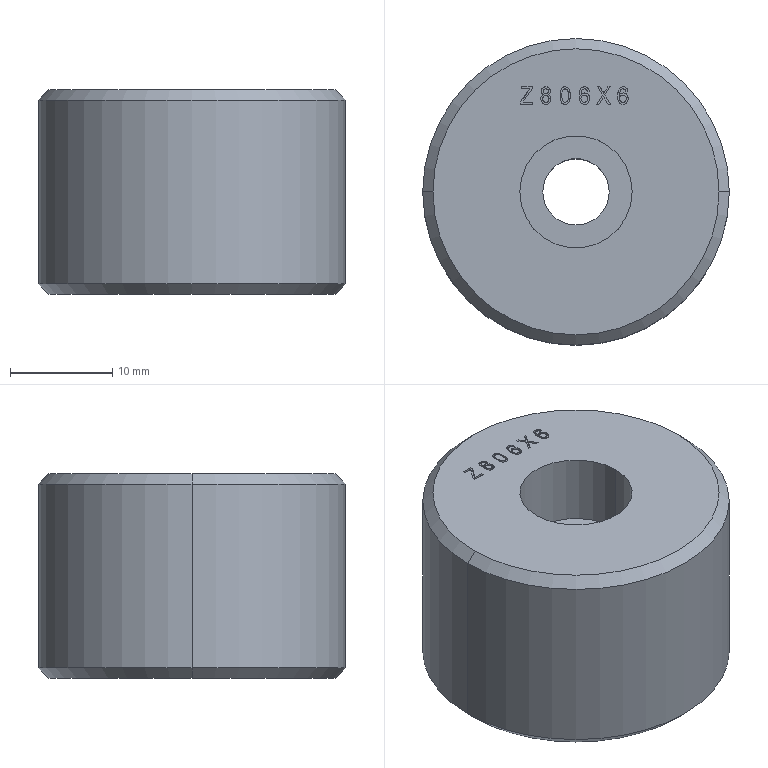Part | Creo | 1 solid | 161 faces | box 30 x 30 x 20 mm | volume 12947 mm3 | other 121 | plane 28 | cylinder 8 | cone 4 | commonest cylinder face diameters 6.5 x2 11 x2 30 x2 0.843 x1 23.072 x1